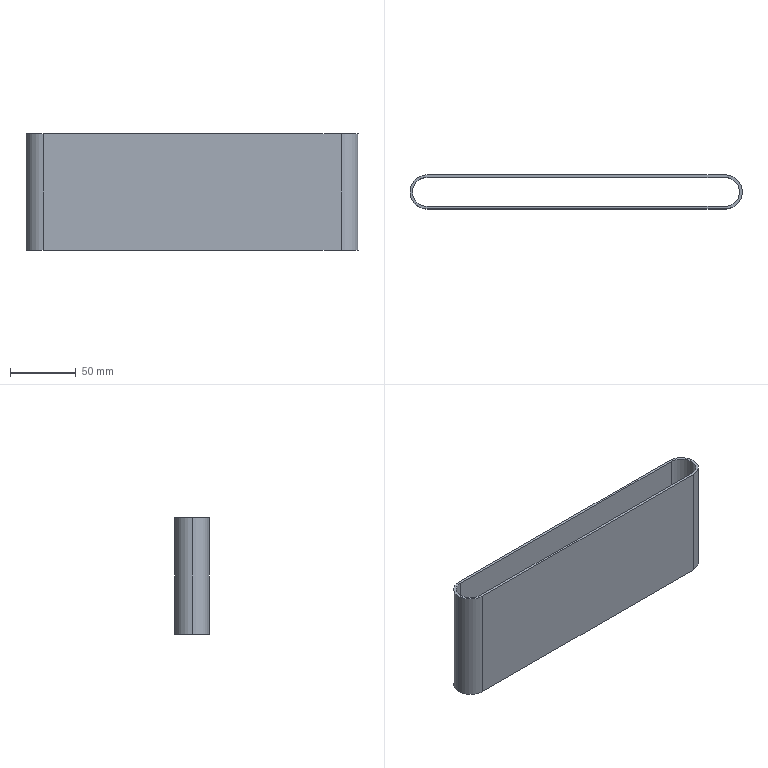Part | STEP file | Green flat belt 477 | 1 solid | 12 faces | box 253 x 26 x 89 mm | volume 94233 mm3 | cylinder 6 | plane 6 | commonest cylinder face diameters 22 x3 26 x3
STEP:
#1=CARTESIAN_POINT('',(-113.5,11.,89.));
#2=VERTEX_POINT('',#1);
#3=CARTESIAN_POINT('',(-124.5,0.,89.));
#4=VERTEX_POINT('',#3);
#5=CARTESIAN_POINT('',(-113.5,0.,89.));
#6=DIRECTION('',(0.,0.,1.));
#7=DIRECTION('',(1.,0.,0.));
#8=AXIS2_PLACEMENT_3D('',#5,#6,#7);
#9=CIRCLE('',#8,11.);
#10=EDGE_CURVE('',#2,#4,#9,.T.);
#11=ORIENTED_EDGE('',*,*,#10,.T.);
#12=CARTESIAN_POINT('',(-124.5,0.,0.));
#13=VERTEX_POINT('',#12);
#14=CARTESIAN_POINT('',(-124.5,0.,89.));
#15=DIRECTION('',(0.,0.,-1.));
#16=VECTOR('',#15,1000.);
#17=LINE('',#14,#16);
#18=EDGE_CURVE('',#4,#13,#17,.T.);
#19=ORIENTED_EDGE('',*,*,#18,.T.);
#20=CARTESIAN_POINT('',(-113.5,11.,0.));
#21=VERTEX_POINT('',#20);
#22=CARTESIAN_POINT('',(-113.5,0.,0.));
#23=DIRECTION('',(0.,0.,1.));
#24=DIRECTION('',(1.,0.,0.));
#25=AXIS2_PLACEMENT_3D('',#22,#23,#24);
#26=CIRCLE('',#25,11.);
#27=EDGE_CURVE('',#21,#13,#26,.T.);
#28=ORIENTED_EDGE('',*,*,#27,.F.);
#29=CARTESIAN_POINT('',(-113.5,11.,89.));
#30=DIRECTION('',(0.,0.,-1.));
#31=VECTOR('',#30,1000.);
#32=LINE('',#29,#31);
#33=EDGE_CURVE('',#2,#21,#32,.T.);
#34=ORIENTED_EDGE('',*,*,#33,.F.);
#35=EDGE_LOOP('',(#11,#19,#28,#34));
#36=FACE_OUTER_BOUND('',#35,.T.);
#37=CARTESIAN_POINT('',(-113.5,0.,89.));
#38=DIRECTION('',(0.,0.,-1.));
#39=DIRECTION('',(-1.,0.,0.));
#40=AXIS2_PLACEMENT_3D('',#37,#38,#39);
#41=CYLINDRICAL_SURFACE('',#40,11.);
#42=ADVANCED_FACE('',(#36),#41,.F.);
#43=CARTESIAN_POINT('',(-126.5,0.,89.));
#44=VERTEX_POINT('',#43);
#45=CARTESIAN_POINT('',(-113.5,-13.,89.));
#46=VERTEX_POINT('',#45);
#47=CARTESIAN_POINT('',(-113.5,0.,89.));
#48=DIRECTION('',(0.,0.,1.));
#49=DIRECTION('',(1.,0.,0.));
#50=AXIS2_PLACEMENT_3D('',#47,#48,#49);
#51=CIRCLE('',#50,13.);
#52=EDGE_CURVE('',#44,#46,#51,.T.);
#53=ORIENTED_EDGE('',*,*,#52,.F.);
#54=CARTESIAN_POINT('',(-126.5,0.,0.));
#55=VERTEX_POINT('',#54);
#56=CARTESIAN_POINT('',(-126.5,0.,89.));
#57=DIRECTION('',(0.,0.,-1.));
#58=VECTOR('',#57,1000.);
#59=LINE('',#56,#58);
#60=EDGE_CURVE('',#44,#55,#59,.T.);
#61=ORIENTED_EDGE('',*,*,#60,.T.);
#62=CARTESIAN_POINT('',(-113.5,-13.,0.));
#63=VERTEX_POINT('',#62);
#64=CARTESIAN_POINT('',(-113.5,0.,0.));
#65=DIRECTION('',(0.,0.,1.));
#66=DIRECTION('',(1.,0.,0.));
#67=AXIS2_PLACEMENT_3D('',#64,#65,#66);
#68=CIRCLE('',#67,13.);
#69=EDGE_CURVE('',#55,#63,#68,.T.);
#70=ORIENTED_EDGE('',*,*,#69,.T.);
#71=CARTESIAN_POINT('',(-113.5,-13.,89.));
#72=DIRECTION('',(0.,0.,-1.));
#73=VECTOR('',#72,1000.);
#74=LINE('',#71,#73);
#75=EDGE_CURVE('',#46,#63,#74,.T.);
#76=ORIENTED_EDGE('',*,*,#75,.F.);
#77=EDGE_LOOP('',(#53,#61,#70,#76));
#78=FACE_OUTER_BOUND('',#77,.T.);
#79=CARTESIAN_POINT('',(-113.5,0.,89.));
#80=DIRECTION('',(0.,0.,-1.));
#81=DIRECTION('',(-1.,0.,0.));
#82=AXIS2_PLACEMENT_3D('',#79,#80,#81);
#83=CYLINDRICAL_SURFACE('',#82,13.);
#84=ADVANCED_FACE('',(#78),#83,.T.);
#85=CARTESIAN_POINT('',(-113.5,13.,89.));
#86=VERTEX_POINT('',#85);
#87=CARTESIAN_POINT('',(-113.5,0.,89.));
#88=DIRECTION('',(0.,0.,1.));
#89=DIRECTION('',(1.,0.,0.));
#90=AXIS2_PLACEMENT_3D('',#87,#88,#89);
#91=CIRCLE('',#90,13.);
#92=EDGE_CURVE('',#86,#44,#91,.T.);
#93=ORIENTED_EDGE('',*,*,#92,.T.);
#94=ORIENTED_EDGE('',*,*,#52,.T.);
#95=CARTESIAN_POINT('',(113.5,-13.,89.));
#96=VERTEX_POINT('',#95);
#97=CARTESIAN_POINT('',(-113.5,-13.,89.));
#98=DIRECTION('',(1.,0.,0.));
#99=VECTOR('',#98,1000.);
#100=LINE('',#97,#99);
#101=EDGE_CURVE('',#46,#96,#100,.T.);
#102=ORIENTED_EDGE('',*,*,#101,.T.);
#103=CARTESIAN_POINT('',(113.5,13.,89.));
#104=VERTEX_POINT('',#103);
#105=CARTESIAN_POINT('',(113.5,0.,89.));
#106=DIRECTION('',(0.,0.,1.));
#107=DIRECTION('',(1.,0.,0.));
#108=AXIS2_PLACEMENT_3D('',#105,#106,#107);
#109=CIRCLE('',#108,13.);
#110=EDGE_CURVE('',#96,#104,#109,.T.);
#111=ORIENTED_EDGE('',*,*,#110,.T.);
#112=CARTESIAN_POINT('',(-113.5,13.,89.));
#113=DIRECTION('',(-1.,0.,0.));
#114=VECTOR('',#113,1000.);
#115=LINE('',#112,#114);
#116=EDGE_CURVE('',#104,#86,#115,.T.);
#117=ORIENTED_EDGE('',*,*,#116,.T.);
#118=EDGE_LOOP('',(#93,#94,#102,#111,#117));
#119=FACE_OUTER_BOUND('',#118,.T.);
#120=CARTESIAN_POINT('',(-113.5,-11.,89.));
#121=VERTEX_POINT('',#120);
#122=CARTESIAN_POINT('',(113.5,-11.,89.));
#123=VERTEX_POINT('',#122);
#124=CARTESIAN_POINT('',(-113.5,-11.,89.));
#125=DIRECTION('',(1.,0.,0.));
#126=VECTOR('',#125,1000.);
#127=LINE('',#124,#126);
#128=EDGE_CURVE('',#121,#123,#127,.T.);
#129=ORIENTED_EDGE('',*,*,#128,.F.);
#130=CARTESIAN_POINT('',(-113.5,0.,89.));
#131=DIRECTION('',(0.,0.,1.));
#132=DIRECTION('',(1.,0.,0.));
#133=AXIS2_PLACEMENT_3D('',#130,#131,#132);
#134=CIRCLE('',#133,11.);
#135=EDGE_CURVE('',#4,#121,#134,.T.);
#136=ORIENTED_EDGE('',*,*,#135,.F.);
#137=ORIENTED_EDGE('',*,*,#10,.F.);
#138=CARTESIAN_POINT('',(113.5,11.,89.));
#139=VERTEX_POINT('',#138);
#140=CARTESIAN_POINT('',(-113.5,11.,89.));
#141=DIRECTION('',(-1.,0.,0.));
#142=VECTOR('',#141,1000.);
#143=LINE('',#140,#142);
#144=EDGE_CURVE('',#139,#2,#143,.T.);
#145=ORIENTED_EDGE('',*,*,#144,.F.);
#146=CARTESIAN_POINT('',(113.5,0.,89.));
#147=DIRECTION('',(0.,0.,1.));
#148=DIRECTION('',(1.,0.,0.));
#149=AXIS2_PLACEMENT_3D('',#146,#147,#148);
#150=CIRCLE('',#149,11.);
#151=EDGE_CURVE('',#123,#139,#150,.T.);
#152=ORIENTED_EDGE('',*,*,#151,.F.);
#153=EDGE_LOOP('',(#129,#136,#137,#145,#152));
#154=FACE_BOUND('',#153,.T.);
#155=CARTESIAN_POINT('',(-113.5,0.,89.));
#156=DIRECTION('',(0.,0.,1.));
#157=DIRECTION('',(1.,0.,0.));
#158=AXIS2_PLACEMENT_3D('',#155,#156,#157);
#159=PLANE('',#158);
#160=ADVANCED_FACE('',(#119,#154),#159,.T.);
#161=CARTESIAN_POINT('',(-113.5,13.,0.));
#162=VERTEX_POINT('',#161);
#163=CARTESIAN_POINT('',(-113.5,0.,0.));
#164=DIRECTION('',(0.,0.,1.));
#165=DIRECTION('',(1.,0.,0.));
#166=AXIS2_PLACEMENT_3D('',#163,#164,#165);
#167=CIRCLE('',#166,13.);
#168=EDGE_CURVE('',#162,#55,#167,.T.);
#169=ORIENTED_EDGE('',*,*,#168,.F.);
#170=CARTESIAN_POINT('',(113.5,13.,0.));
#171=VERTEX_POINT('',#170);
#172=CARTESIAN_POINT('',(-113.5,13.,0.));
#173=DIRECTION('',(-1.,0.,0.));
#174=VECTOR('',#173,1000.);
#175=LINE('',#172,#174);
#176=EDGE_CURVE('',#171,#162,#175,.T.);
#177=ORIENTED_EDGE('',*,*,#176,.F.);
#178=CARTESIAN_POINT('',(113.5,-13.,0.));
#179=VERTEX_POINT('',#178);
#180=CARTESIAN_POINT('',(113.5,0.,0.));
#181=DIRECTION('',(0.,0.,1.));
#182=DIRECTION('',(1.,0.,0.));
#183=AXIS2_PLACEMENT_3D('',#180,#181,#182);
#184=CIRCLE('',#183,13.);
#185=EDGE_CURVE('',#179,#171,#184,.T.);
#186=ORIENTED_EDGE('',*,*,#185,.F.);
#187=CARTESIAN_POINT('',(-113.5,-13.,0.));
#188=DIRECTION('',(1.,0.,0.));
#189=VECTOR('',#188,1000.);
#190=LINE('',#187,#189);
#191=EDGE_CURVE('',#63,#179,#190,.T.);
#192=ORIENTED_EDGE('',*,*,#191,.F.);
#193=ORIENTED_EDGE('',*,*,#69,.F.);
#194=EDGE_LOOP('',(#169,#177,#186,#192,#193));
#195=FACE_OUTER_BOUND('',#194,.T.);
#196=ORIENTED_EDGE('',*,*,#27,.T.);
#197=CARTESIAN_POINT('',(-113.5,-11.,0.));
#198=VERTEX_POINT('',#197);
#199=CARTESIAN_POINT('',(-113.5,0.,0.));
#200=DIRECTION('',(0.,0.,1.));
#201=DIRECTION('',(1.,0.,0.));
#202=AXIS2_PLACEMENT_3D('',#199,#200,#201);
#203=CIRCLE('',#202,11.);
#204=EDGE_CURVE('',#13,#198,#203,.T.);
#205=ORIENTED_EDGE('',*,*,#204,.T.);
#206=CARTESIAN_POINT('',(113.5,-11.,0.));
#207=VERTEX_POINT('',#206);
#208=CARTESIAN_POINT('',(-113.5,-11.,0.));
#209=DIRECTION('',(1.,0.,0.));
#210=VECTOR('',#209,1000.);
#211=LINE('',#208,#210);
#212=EDGE_CURVE('',#198,#207,#211,.T.);
#213=ORIENTED_EDGE('',*,*,#212,.T.);
#214=CARTESIAN_POINT('',(113.5,11.,0.));
#215=VERTEX_POINT('',#214);
#216=CARTESIAN_POINT('',(113.5,0.,0.));
#217=DIRECTION('',(0.,0.,1.));
#218=DIRECTION('',(1.,0.,0.));
#219=AXIS2_PLACEMENT_3D('',#216,#217,#218);
#220=CIRCLE('',#219,11.);
#221=EDGE_CURVE('',#207,#215,#220,.T.);
#222=ORIENTED_EDGE('',*,*,#221,.T.);
#223=CARTESIAN_POINT('',(-113.5,11.,0.));
#224=DIRECTION('',(-1.,0.,0.));
#225=VECTOR('',#224,1000.);
#226=LINE('',#223,#225);
#227=EDGE_CURVE('',#215,#21,#226,.T.);
#228=ORIENTED_EDGE('',*,*,#227,.T.);
#229=EDGE_LOOP('',(#196,#205,#213,#222,#228));
#230=FACE_BOUND('',#229,.T.);
#231=CARTESIAN_POINT('',(-113.5,0.,0.));
#232=DIRECTION('',(0.,0.,1.));
#233=DIRECTION('',(1.,0.,0.));
#234=AXIS2_PLACEMENT_3D('',#231,#232,#233);
#235=PLANE('',#234);
#236=ADVANCED_FACE('',(#195,#230),#235,.F.);
#237=ORIENTED_EDGE('',*,*,#60,.F.);
#238=ORIENTED_EDGE('',*,*,#92,.F.);
#239=CARTESIAN_POINT('',(-113.5,13.,89.));
#240=DIRECTION('',(0.,0.,-1.));
#241=VECTOR('',#240,1000.);
#242=LINE('',#239,#241);
#243=EDGE_CURVE('',#86,#162,#242,.T.);
#244=ORIENTED_EDGE('',*,*,#243,.T.);
#245=ORIENTED_EDGE('',*,*,#168,.T.);
#246=EDGE_LOOP('',(#237,#238,#244,#245));
#247=FACE_OUTER_BOUND('',#246,.T.);
#248=CARTESIAN_POINT('',(-113.5,0.,89.));
#249=DIRECTION('',(0.,0.,-1.));
#250=DIRECTION('',(-1.,0.,0.));
#251=AXIS2_PLACEMENT_3D('',#248,#249,#250);
#252=CYLINDRICAL_SURFACE('',#251,13.);
#253=ADVANCED_FACE('',(#247),#252,.T.);
#254=ORIENTED_EDGE('',*,*,#191,.T.);
#255=CARTESIAN_POINT('',(113.5,-13.,89.));
#256=DIRECTION('',(0.,0.,-1.));
#257=VECTOR('',#256,1000.);
#258=LINE('',#255,#257);
#259=EDGE_CURVE('',#96,#179,#258,.T.);
#260=ORIENTED_EDGE('',*,*,#259,.F.);
#261=ORIENTED_EDGE('',*,*,#101,.F.);
#262=ORIENTED_EDGE('',*,*,#75,.T.);
#263=EDGE_LOOP('',(#254,#260,#261,#262));
#264=FACE_OUTER_BOUND('',#263,.T.);
#265=CARTESIAN_POINT('',(-113.5,-13.,89.));
#266=DIRECTION('',(0.,1.,0.));
#267=DIRECTION('',(-1.,0.,0.));
#268=AXIS2_PLACEMENT_3D('',#265,#266,#267);
#269=PLANE('',#268);
#270=ADVANCED_FACE('',(#264),#269,.F.);
#271=ORIENTED_EDGE('',*,*,#185,.T.);
#272=CARTESIAN_POINT('',(113.5,13.,89.));
#273=DIRECTION('',(0.,0.,-1.));
#274=VECTOR('',#273,1000.);
#275=LINE('',#272,#274);
#276=EDGE_CURVE('',#104,#171,#275,.T.);
#277=ORIENTED_EDGE('',*,*,#276,.F.);
#278=ORIENTED_EDGE('',*,*,#110,.F.);
#279=ORIENTED_EDGE('',*,*,#259,.T.);
#280=EDGE_LOOP('',(#271,#277,#278,#279));
#281=FACE_OUTER_BOUND('',#280,.T.);
#282=CARTESIAN_POINT('',(113.5,0.,89.));
#283=DIRECTION('',(0.,0.,-1.));
#284=DIRECTION('',(-1.,0.,0.));
#285=AXIS2_PLACEMENT_3D('',#282,#283,#284);
#286=CYLINDRICAL_SURFACE('',#285,13.);
#287=ADVANCED_FACE('',(#281),#286,.T.);
#288=ORIENTED_EDGE('',*,*,#176,.T.);
#289=ORIENTED_EDGE('',*,*,#243,.F.);
#290=ORIENTED_EDGE('',*,*,#116,.F.);
#291=ORIENTED_EDGE('',*,*,#276,.T.);
#292=EDGE_LOOP('',(#288,#289,#290,#291));
#293=FACE_OUTER_BOUND('',#292,.T.);
#294=CARTESIAN_POINT('',(-113.5,13.,89.));
#295=DIRECTION('',(0.,-1.,0.));
#296=DIRECTION('',(0.,0.,-1.));
#297=AXIS2_PLACEMENT_3D('',#294,#295,#296);
#298=PLANE('',#297);
#299=ADVANCED_FACE('',(#293),#298,.F.);
#300=ORIENTED_EDGE('',*,*,#18,.F.);
#301=ORIENTED_EDGE('',*,*,#135,.T.);
#302=CARTESIAN_POINT('',(-113.5,-11.,89.));
#303=DIRECTION('',(0.,0.,-1.));
#304=VECTOR('',#303,1000.);
#305=LINE('',#302,#304);
#306=EDGE_CURVE('',#121,#198,#305,.T.);
#307=ORIENTED_EDGE('',*,*,#306,.T.);
#308=ORIENTED_EDGE('',*,*,#204,.F.);
#309=EDGE_LOOP('',(#300,#301,#307,#308));
#310=FACE_OUTER_BOUND('',#309,.T.);
#311=CARTESIAN_POINT('',(-113.5,0.,89.));
#312=DIRECTION('',(0.,0.,-1.));
#313=DIRECTION('',(-1.,0.,0.));
#314=AXIS2_PLACEMENT_3D('',#311,#312,#313);
#315=CYLINDRICAL_SURFACE('',#314,11.);
#316=ADVANCED_FACE('',(#310),#315,.F.);
#317=ORIENTED_EDGE('',*,*,#212,.F.);
#318=ORIENTED_EDGE('',*,*,#306,.F.);
#319=ORIENTED_EDGE('',*,*,#128,.T.);
#320=CARTESIAN_POINT('',(113.5,-11.,89.));
#321=DIRECTION('',(0.,0.,-1.));
#322=VECTOR('',#321,1000.);
#323=LINE('',#320,#322);
#324=EDGE_CURVE('',#123,#207,#323,.T.);
#325=ORIENTED_EDGE('',*,*,#324,.T.);
#326=EDGE_LOOP('',(#317,#318,#319,#325));
#327=FACE_OUTER_BOUND('',#326,.T.);
#328=CARTESIAN_POINT('',(-113.5,-11.,89.));
#329=DIRECTION('',(0.,1.,0.));
#330=DIRECTION('',(-1.,0.,0.));
#331=AXIS2_PLACEMENT_3D('',#328,#329,#330);
#332=PLANE('',#331);
#333=ADVANCED_FACE('',(#327),#332,.T.);
#334=ORIENTED_EDGE('',*,*,#221,.F.);
#335=ORIENTED_EDGE('',*,*,#324,.F.);
#336=ORIENTED_EDGE('',*,*,#151,.T.);
#337=CARTESIAN_POINT('',(113.5,11.,89.));
#338=DIRECTION('',(0.,0.,-1.));
#339=VECTOR('',#338,1000.);
#340=LINE('',#337,#339);
#341=EDGE_CURVE('',#139,#215,#340,.T.);
#342=ORIENTED_EDGE('',*,*,#341,.T.);
#343=EDGE_LOOP('',(#334,#335,#336,#342));
#344=FACE_OUTER_BOUND('',#343,.T.);
#345=CARTESIAN_POINT('',(113.5,0.,89.));
#346=DIRECTION('',(0.,0.,-1.));
#347=DIRECTION('',(-1.,0.,0.));
#348=AXIS2_PLACEMENT_3D('',#345,#346,#347);
#349=CYLINDRICAL_SURFACE('',#348,11.);
#350=ADVANCED_FACE('',(#344),#349,.F.);
#351=ORIENTED_EDGE('',*,*,#227,.F.);
#352=ORIENTED_EDGE('',*,*,#341,.F.);
#353=ORIENTED_EDGE('',*,*,#144,.T.);
#354=ORIENTED_EDGE('',*,*,#33,.T.);
#355=EDGE_LOOP('',(#351,#352,#353,#354));
#356=FACE_OUTER_BOUND('',#355,.T.);
#357=CARTESIAN_POINT('',(-113.5,11.,89.));
#358=DIRECTION('',(0.,-1.,0.));
#359=DIRECTION('',(1.,0.,0.));
#360=AXIS2_PLACEMENT_3D('',#357,#358,#359);
#361=PLANE('',#360);
#362=ADVANCED_FACE('',(#356),#361,.T.);
#363=CLOSED_SHELL('',(#42,#84,#160,#236,#253,#270,#287,#299,#316,#333,#350,#362));
#364=MANIFOLD_SOLID_BREP('',#363);
#365=CARTESIAN_POINT('',(0.,0.,0.));
#366=DIRECTION('',(0.,0.,1.));
#367=DIRECTION('',(1.,0.,0.));
#368=AXIS2_PLACEMENT_3D('',#365,#366,#367);
#369=(LENGTH_UNIT()NAMED_UNIT(*)SI_UNIT(.MILLI.,.METRE.));
#370=UNCERTAINTY_MEASURE_WITH_UNIT(LENGTH_MEASURE(0.00001),#369,'','');
#371=(NAMED_UNIT(*)PLANE_ANGLE_UNIT()SI_UNIT($,.RADIAN.));
#372=(NAMED_UNIT(*)SI_UNIT($,.STERADIAN.)SOLID_ANGLE_UNIT());
#373=(GEOMETRIC_REPRESENTATION_CONTEXT(3)GLOBAL_UNCERTAINTY_ASSIGNED_CONTEXT((#370))GLOBAL_UNIT_ASSIGNED_CONTEXT((#369,#371,#372))REPRESENTATION_CONTEXT('',''));
#374=ADVANCED_BREP_SHAPE_REPRESENTATION('',(#364,#368),#373);